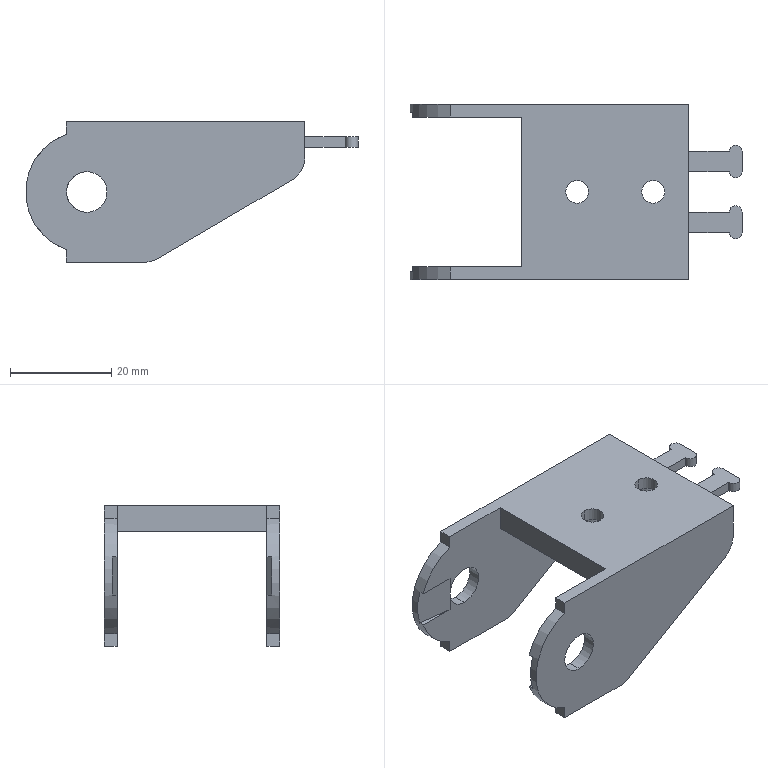Part | NX | features BREP 1 | 1 solid | 52 faces | box 65.5 x 34.5 x 27.7 mm | volume 10299 mm3 | plane 30 | cylinder 18 | cone 4 | commonest cylinder face diameters 2.5 x4 4.5 x4 8 x4 10 x4 24.103 x2